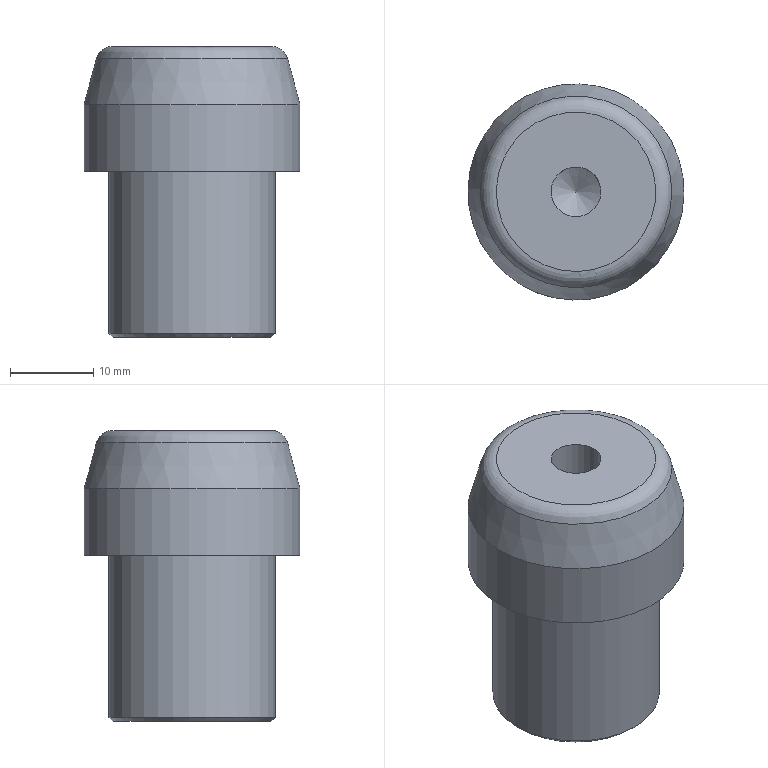Part | NX | features solid 2 | 1 solid | 10 faces | box 26 x 26 x 35 mm | volume 13398 mm3 | plane 3 | cylinder 3 | cone 3 | torus 1 | commonest cylinder face diameters 6 x1 20 x1 26 x1
STEP:
#1=CARTESIAN_POINT('',(643.251,-11.286,161.));
#2=VERTEX_POINT('',#1);
#3=CARTESIAN_POINT('',(653.247,-11.594,161.));
#4=DIRECTION('',(0.,0.,-1.));
#5=DIRECTION('',(-0.9995,0.0308,0.));
#6=AXIS2_PLACEMENT_3D('',#3,#4,#5);
#7=CIRCLE('',#6,10.);
#8=EDGE_CURVE('',#2,#2,#7,.T.);
#9=ORIENTED_EDGE('',*,*,#8,.F.);
#10=EDGE_LOOP('',(#9));
#11=FACE_BOUND('',#10,.T.);
#12=CARTESIAN_POINT('',(666.241,-11.994,161.));
#13=VERTEX_POINT('',#12);
#14=CARTESIAN_POINT('',(653.247,-11.594,161.));
#15=DIRECTION('',(0.,0.,1.));
#16=DIRECTION('',(0.9995,-0.0308,0.));
#17=AXIS2_PLACEMENT_3D('',#14,#15,#16);
#18=CIRCLE('',#17,13.);
#19=EDGE_CURVE('',#13,#13,#18,.T.);
#20=ORIENTED_EDGE('',*,*,#19,.F.);
#21=EDGE_LOOP('',(#20));
#22=FACE_BOUND('',#21,.T.);
#23=CARTESIAN_POINT('',(653.247,-11.594,161.));
#24=DIRECTION('',(0.,0.,-1.));
#25=DIRECTION('',(-0.9995,0.0308,0.));
#26=AXIS2_PLACEMENT_3D('',#23,#24,#25);
#27=PLANE('',#26);
#28=ADVANCED_FACE('',(#11,#22),#27,.T.);
#29=CARTESIAN_POINT('',(640.253,-11.193,169.));
#30=VERTEX_POINT('',#29);
#31=CARTESIAN_POINT('',(653.247,-11.594,169.));
#32=DIRECTION('',(0.,0.,-1.));
#33=DIRECTION('',(-0.9995,0.0308,0.));
#34=AXIS2_PLACEMENT_3D('',#31,#32,#33);
#35=CIRCLE('',#34,13.);
#36=EDGE_CURVE('',#30,#30,#35,.T.);
#37=ORIENTED_EDGE('',*,*,#36,.T.);
#38=EDGE_LOOP('',(#37));
#39=FACE_BOUND('',#38,.T.);
#40=ORIENTED_EDGE('',*,*,#19,.T.);
#41=EDGE_LOOP('',(#40));
#42=FACE_BOUND('',#41,.T.);
#43=CARTESIAN_POINT('',(653.247,-11.594,161.));
#44=DIRECTION('',(0.,0.,1.));
#45=DIRECTION('',(0.9995,-0.0308,0.));
#46=AXIS2_PLACEMENT_3D('',#43,#44,#45);
#47=CYLINDRICAL_SURFACE('',#46,13.);
#48=ADVANCED_FACE('',(#39,#42),#47,.T.);
#49=CARTESIAN_POINT('',(641.731,-11.239,174.518));
#50=VERTEX_POINT('',#49);
#51=CARTESIAN_POINT('',(653.247,-11.594,174.518));
#52=DIRECTION('',(0.,0.,-1.));
#53=DIRECTION('',(-0.9995,0.0308,0.));
#54=AXIS2_PLACEMENT_3D('',#51,#52,#53);
#55=CIRCLE('',#54,11.522);
#56=EDGE_CURVE('',#50,#50,#55,.T.);
#57=ORIENTED_EDGE('',*,*,#56,.T.);
#58=EDGE_LOOP('',(#57));
#59=FACE_BOUND('',#58,.T.);
#60=ORIENTED_EDGE('',*,*,#36,.F.);
#61=EDGE_LOOP('',(#60));
#62=FACE_BOUND('',#61,.T.);
#63=CARTESIAN_POINT('',(653.247,-11.594,169.));
#64=DIRECTION('',(0.,0.,-1.));
#65=DIRECTION('',(0.9995,-0.0308,0.));
#66=AXIS2_PLACEMENT_3D('',#63,#64,#65);
#67=CONICAL_SURFACE('',#66,13.,0.2618);
#68=ADVANCED_FACE('',(#59,#62),#67,.T.);
#69=CARTESIAN_POINT('',(650.248,-11.501,176.));
#70=VERTEX_POINT('',#69);
#71=CARTESIAN_POINT('',(653.247,-11.594,176.));
#72=DIRECTION('',(0.,0.,-1.));
#73=DIRECTION('',(-0.9995,0.0308,0.));
#74=AXIS2_PLACEMENT_3D('',#71,#72,#73);
#75=CIRCLE('',#74,3.);
#76=EDGE_CURVE('',#70,#70,#75,.T.);
#77=ORIENTED_EDGE('',*,*,#76,.T.);
#78=EDGE_LOOP('',(#77));
#79=FACE_BOUND('',#78,.T.);
#80=CARTESIAN_POINT('',(643.662,-11.298,176.));
#81=VERTEX_POINT('',#80);
#82=CARTESIAN_POINT('',(653.247,-11.594,176.));
#83=DIRECTION('',(0.,0.,-1.));
#84=DIRECTION('',(-0.9995,0.0308,0.));
#85=AXIS2_PLACEMENT_3D('',#82,#83,#84);
#86=CIRCLE('',#85,9.59);
#87=EDGE_CURVE('',#81,#81,#86,.F.);
#88=ORIENTED_EDGE('',*,*,#87,.T.);
#89=EDGE_LOOP('',(#88));
#90=FACE_BOUND('',#89,.T.);
#91=CARTESIAN_POINT('',(653.247,-11.594,176.));
#92=DIRECTION('',(0.,0.,-1.));
#93=DIRECTION('',(-0.9995,0.0308,0.));
#94=AXIS2_PLACEMENT_3D('',#91,#92,#93);
#95=PLANE('',#94);
#96=ADVANCED_FACE('',(#79,#90),#95,.F.);
#97=CARTESIAN_POINT('',(643.751,-11.301,141.));
#98=VERTEX_POINT('',#97);
#99=CARTESIAN_POINT('',(653.247,-11.594,141.));
#100=DIRECTION('',(0.,0.,-1.));
#101=DIRECTION('',(-0.9995,0.0308,0.));
#102=AXIS2_PLACEMENT_3D('',#99,#100,#101);
#103=CIRCLE('',#102,9.5);
#104=EDGE_CURVE('',#98,#98,#103,.T.);
#105=ORIENTED_EDGE('',*,*,#104,.T.);
#106=EDGE_LOOP('',(#105));
#107=FACE_BOUND('',#106,.T.);
#108=CARTESIAN_POINT('',(653.247,-11.594,141.));
#109=DIRECTION('',(0.,0.,-1.));
#110=DIRECTION('',(-0.9995,0.0308,0.));
#111=AXIS2_PLACEMENT_3D('',#108,#109,#110);
#112=PLANE('',#111);
#113=ADVANCED_FACE('',(#107),#112,.T.);
#114=CARTESIAN_POINT('',(643.251,-11.286,141.5));
#115=VERTEX_POINT('',#114);
#116=CARTESIAN_POINT('',(653.247,-11.594,141.5));
#117=DIRECTION('',(0.,0.,-1.));
#118=DIRECTION('',(-0.9995,0.0308,0.));
#119=AXIS2_PLACEMENT_3D('',#116,#117,#118);
#120=CIRCLE('',#119,10.);
#121=EDGE_CURVE('',#115,#115,#120,.F.);
#122=ORIENTED_EDGE('',*,*,#121,.T.);
#123=EDGE_LOOP('',(#122));
#124=FACE_BOUND('',#123,.T.);
#125=ORIENTED_EDGE('',*,*,#8,.T.);
#126=EDGE_LOOP('',(#125));
#127=FACE_BOUND('',#126,.T.);
#128=CARTESIAN_POINT('',(653.247,-11.594,161.));
#129=DIRECTION('',(0.,0.,-1.));
#130=DIRECTION('',(-0.9995,0.0308,0.));
#131=AXIS2_PLACEMENT_3D('',#128,#129,#130);
#132=CYLINDRICAL_SURFACE('',#131,10.);
#133=ADVANCED_FACE('',(#124,#127),#132,.T.);
#134=ORIENTED_EDGE('',*,*,#121,.F.);
#135=EDGE_LOOP('',(#134));
#136=FACE_BOUND('',#135,.T.);
#137=ORIENTED_EDGE('',*,*,#104,.F.);
#138=EDGE_LOOP('',(#137));
#139=FACE_BOUND('',#138,.T.);
#140=CARTESIAN_POINT('',(653.247,-11.594,141.));
#141=DIRECTION('',(0.,0.,1.));
#142=DIRECTION('',(0.9995,-0.0308,0.));
#143=AXIS2_PLACEMENT_3D('',#140,#141,#142);
#144=CONICAL_SURFACE('',#143,9.5,0.7854);
#145=ADVANCED_FACE('',(#136,#139),#144,.T.);
#146=ORIENTED_EDGE('',*,*,#87,.F.);
#147=EDGE_LOOP('',(#146));
#148=FACE_BOUND('',#147,.T.);
#149=ORIENTED_EDGE('',*,*,#56,.F.);
#150=EDGE_LOOP('',(#149));
#151=FACE_BOUND('',#150,.T.);
#152=CARTESIAN_POINT('',(653.247,-11.594,174.));
#153=DIRECTION('',(0.,0.,-1.));
#154=DIRECTION('',(-0.9995,0.0308,0.));
#155=AXIS2_PLACEMENT_3D('',#152,#153,#154);
#156=TOROIDAL_SURFACE('',#155,9.59,2.);
#157=ADVANCED_FACE('',(#148,#151),#156,.T.);
#158=CARTESIAN_POINT('',(650.248,-11.501,166.));
#159=VERTEX_POINT('',#158);
#160=CARTESIAN_POINT('',(653.247,-11.594,166.));
#161=DIRECTION('',(0.,0.,-1.));
#162=DIRECTION('',(-0.9995,0.0308,0.));
#163=AXIS2_PLACEMENT_3D('',#160,#161,#162);
#164=CIRCLE('',#163,3.);
#165=EDGE_CURVE('',#159,#159,#164,.T.);
#166=ORIENTED_EDGE('',*,*,#165,.F.);
#167=EDGE_LOOP('',(#166));
#168=FACE_BOUND('',#167,.T.);
#169=CARTESIAN_POINT('',(653.247,-11.594,164.197));
#170=VERTEX_POINT('',#169);
#171=VERTEX_LOOP('',#170);
#172=FACE_BOUND('',#171,.T.);
#173=CARTESIAN_POINT('',(653.247,-11.594,166.));
#174=DIRECTION('',(0.,0.,1.));
#175=DIRECTION('',(0.9995,-0.0308,0.));
#176=AXIS2_PLACEMENT_3D('',#173,#174,#175);
#177=CONICAL_SURFACE('',#176,3.,1.03);
#178=ADVANCED_FACE('',(#168,#172),#177,.F.);
#179=ORIENTED_EDGE('',*,*,#165,.T.);
#180=EDGE_LOOP('',(#179));
#181=FACE_BOUND('',#180,.T.);
#182=ORIENTED_EDGE('',*,*,#76,.F.);
#183=EDGE_LOOP('',(#182));
#184=FACE_BOUND('',#183,.T.);
#185=CARTESIAN_POINT('',(653.247,-11.594,176.));
#186=DIRECTION('',(0.,0.,-1.));
#187=DIRECTION('',(-0.9995,0.0308,0.));
#188=AXIS2_PLACEMENT_3D('',#185,#186,#187);
#189=CYLINDRICAL_SURFACE('',#188,3.);
#190=ADVANCED_FACE('',(#181,#184),#189,.F.);
#191=CLOSED_SHELL('',(#28,#48,#68,#96,#113,#133,#145,#157,#178,#190));
#192=MANIFOLD_SOLID_BREP('',#191);
#193=(LENGTH_UNIT()NAMED_UNIT(*)SI_UNIT(.MILLI.,.METRE.));
#194=UNCERTAINTY_MEASURE_WITH_UNIT(LENGTH_MEASURE(0.00001),#193,'','');
#195=(NAMED_UNIT(*)PLANE_ANGLE_UNIT()SI_UNIT($,.RADIAN.));
#196=(NAMED_UNIT(*)SI_UNIT($,.STERADIAN.)SOLID_ANGLE_UNIT());
#197=(GEOMETRIC_REPRESENTATION_CONTEXT(3)GLOBAL_UNCERTAINTY_ASSIGNED_CONTEXT((#194))GLOBAL_UNIT_ASSIGNED_CONTEXT((#193,#195,#196))REPRESENTATION_CONTEXT('',''));
#198=ADVANCED_BREP_SHAPE_REPRESENTATION('',(#192),#197);